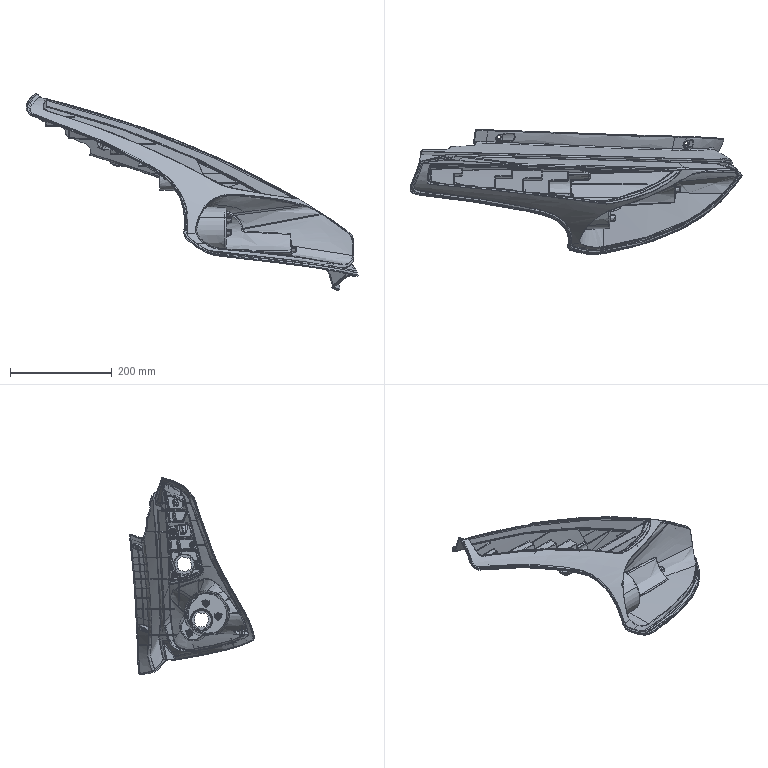Part | STEP file | solid 9 | 1 solid | 1922 faces | box 652.487 x 245.59 x 387.851 mm | volume 665205 mm3 | spline 1415 | plane 222 | sphere 81 | cylinder 78 | cone 61 | torus 55 | other 10 | commonest cylinder face diameters 2.01 x21 4.02 x20 27.135 x8 31.155 x8 2.915 x7 1.005 x6